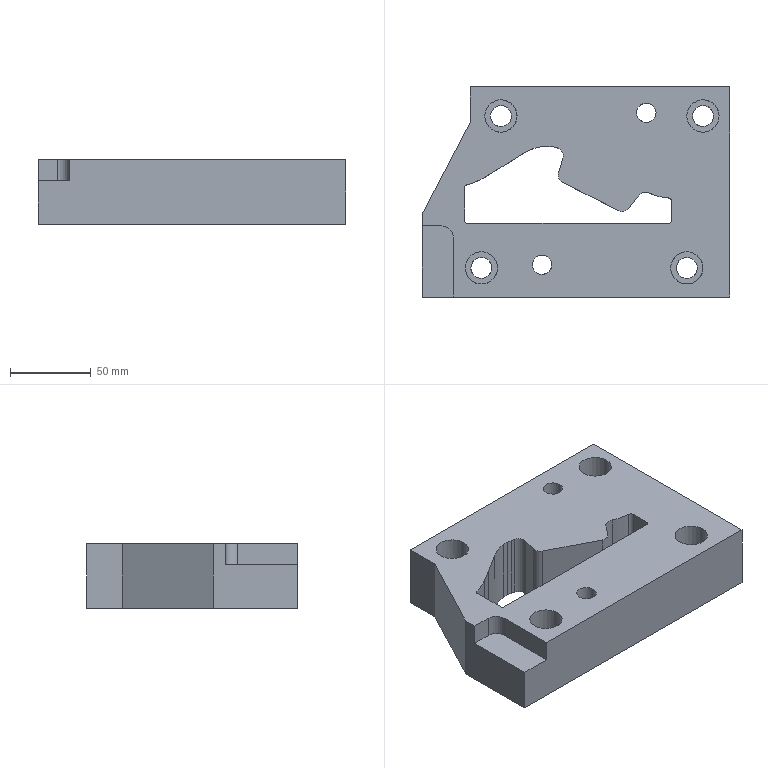Part | STEP file | gslz 2016.10.28-13_id186_x_t | 1 solid | 49 faces | box 190 x 130 x 40 mm | volume 741294 mm3 | plane 26 | cylinder 23 | commonest cylinder face diameters 4 x4 13 x4 20 x4 10 x3 12 x3 14 x1